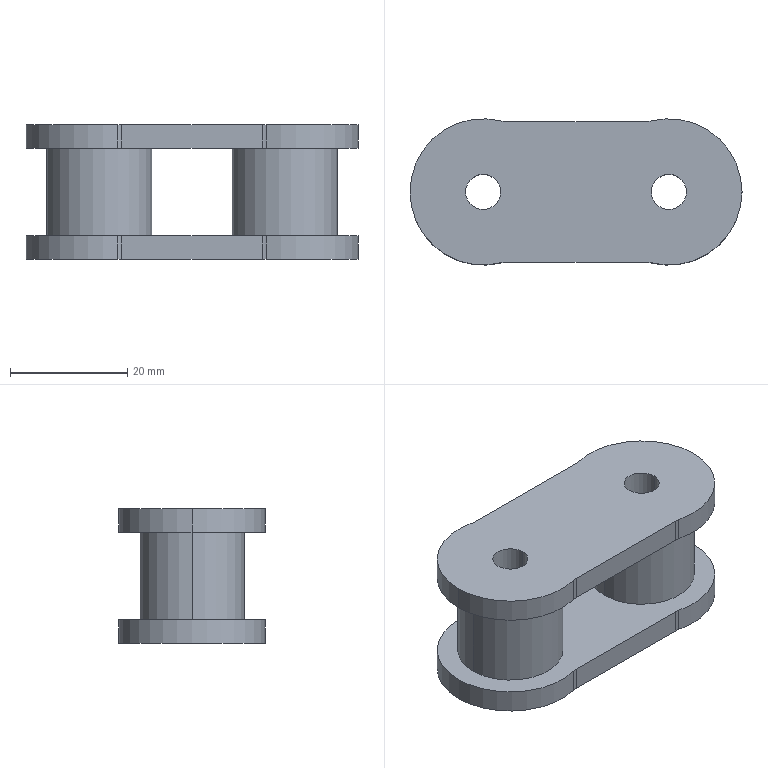Part | STEP file | Motor output chain-06B link 1 | 1 solid | 30 faces | box 56.75 x 25 x 23 mm | volume 16394 mm3 | cylinder 22 | plane 8 | commonest cylinder face diameters 6 x12 25 x6 18 x4
STEP:
#1=CARTESIAN_POINT('',(12.875,0.,-11.5));
#2=VERTEX_POINT('',#1);
#3=CARTESIAN_POINT('',(18.875,0.,-11.5));
#4=VERTEX_POINT('',#3);
#5=CARTESIAN_POINT('',(15.875,0.,-11.5));
#6=DIRECTION('',(0.,0.,1.));
#7=DIRECTION('',(1.,0.,0.));
#8=AXIS2_PLACEMENT_3D('',#5,#6,#7);
#9=CIRCLE('',#8,3.);
#10=EDGE_CURVE('',#2,#4,#9,.T.);
#11=ORIENTED_EDGE('',*,*,#10,.F.);
#12=CARTESIAN_POINT('',(12.875,0.,11.5));
#13=VERTEX_POINT('',#12);
#14=CARTESIAN_POINT('',(12.875,0.,-11.5));
#15=DIRECTION('',(0.,0.,1.));
#16=VECTOR('',#15,1000.);
#17=LINE('',#14,#16);
#18=EDGE_CURVE('',#2,#13,#17,.T.);
#19=ORIENTED_EDGE('',*,*,#18,.T.);
#20=CARTESIAN_POINT('',(18.875,0.,11.5));
#21=VERTEX_POINT('',#20);
#22=CARTESIAN_POINT('',(15.875,0.,11.5));
#23=DIRECTION('',(0.,0.,1.));
#24=DIRECTION('',(1.,0.,0.));
#25=AXIS2_PLACEMENT_3D('',#22,#23,#24);
#26=CIRCLE('',#25,3.);
#27=EDGE_CURVE('',#13,#21,#26,.T.);
#28=ORIENTED_EDGE('',*,*,#27,.T.);
#29=CARTESIAN_POINT('',(18.875,0.,-11.5));
#30=DIRECTION('',(0.,0.,1.));
#31=VECTOR('',#30,1000.);
#32=LINE('',#29,#31);
#33=EDGE_CURVE('',#4,#21,#32,.T.);
#34=ORIENTED_EDGE('',*,*,#33,.F.);
#35=EDGE_LOOP('',(#11,#19,#28,#34));
#36=FACE_OUTER_BOUND('',#35,.T.);
#37=CARTESIAN_POINT('',(15.875,0.,-11.5));
#38=DIRECTION('',(0.,0.,1.));
#39=DIRECTION('',(1.,0.,0.));
#40=AXIS2_PLACEMENT_3D('',#37,#38,#39);
#41=CYLINDRICAL_SURFACE('',#40,3.);
#42=ADVANCED_FACE('',(#36),#41,.F.);
#43=CARTESIAN_POINT('',(-18.875,0.,-11.5));
#44=VERTEX_POINT('',#43);
#45=CARTESIAN_POINT('',(-12.875,0.,-11.5));
#46=VERTEX_POINT('',#45);
#47=CARTESIAN_POINT('',(-15.875,0.,-11.5));
#48=DIRECTION('',(0.,0.,1.));
#49=DIRECTION('',(1.,0.,0.));
#50=AXIS2_PLACEMENT_3D('',#47,#48,#49);
#51=CIRCLE('',#50,3.);
#52=EDGE_CURVE('',#44,#46,#51,.T.);
#53=ORIENTED_EDGE('',*,*,#52,.F.);
#54=CARTESIAN_POINT('',(-18.875,0.,11.5));
#55=VERTEX_POINT('',#54);
#56=CARTESIAN_POINT('',(-18.875,0.,-11.5));
#57=DIRECTION('',(0.,0.,1.));
#58=VECTOR('',#57,1000.);
#59=LINE('',#56,#58);
#60=EDGE_CURVE('',#44,#55,#59,.T.);
#61=ORIENTED_EDGE('',*,*,#60,.T.);
#62=CARTESIAN_POINT('',(-12.875,0.,11.5));
#63=VERTEX_POINT('',#62);
#64=CARTESIAN_POINT('',(-15.875,0.,11.5));
#65=DIRECTION('',(0.,0.,1.));
#66=DIRECTION('',(1.,0.,0.));
#67=AXIS2_PLACEMENT_3D('',#64,#65,#66);
#68=CIRCLE('',#67,3.);
#69=EDGE_CURVE('',#55,#63,#68,.T.);
#70=ORIENTED_EDGE('',*,*,#69,.T.);
#71=CARTESIAN_POINT('',(-12.875,0.,-11.5));
#72=DIRECTION('',(0.,0.,1.));
#73=VECTOR('',#72,1000.);
#74=LINE('',#71,#73);
#75=EDGE_CURVE('',#46,#63,#74,.T.);
#76=ORIENTED_EDGE('',*,*,#75,.F.);
#77=EDGE_LOOP('',(#53,#61,#70,#76));
#78=FACE_OUTER_BOUND('',#77,.T.);
#79=CARTESIAN_POINT('',(-15.875,0.,-11.5));
#80=DIRECTION('',(0.,0.,1.));
#81=DIRECTION('',(1.,0.,0.));
#82=AXIS2_PLACEMENT_3D('',#79,#80,#81);
#83=CYLINDRICAL_SURFACE('',#82,3.);
#84=ADVANCED_FACE('',(#78),#83,.F.);
#85=CARTESIAN_POINT('',(12.726,-12.097,-11.5));
#86=VERTEX_POINT('',#85);
#87=CARTESIAN_POINT('',(28.375,0.,-11.5));
#88=VERTEX_POINT('',#87);
#89=CARTESIAN_POINT('',(15.875,0.,-11.5));
#90=DIRECTION('',(0.,0.,1.));
#91=DIRECTION('',(1.,0.,0.));
#92=AXIS2_PLACEMENT_3D('',#89,#90,#91);
#93=CIRCLE('',#92,12.5);
#94=EDGE_CURVE('',#86,#88,#93,.T.);
#95=ORIENTED_EDGE('',*,*,#94,.T.);
#96=CARTESIAN_POINT('',(28.375,0.,-7.5));
#97=VERTEX_POINT('',#96);
#98=CARTESIAN_POINT('',(28.375,0.,-11.5));
#99=DIRECTION('',(0.,0.,1.));
#100=VECTOR('',#99,1000.);
#101=LINE('',#98,#100);
#102=EDGE_CURVE('',#88,#97,#101,.T.);
#103=ORIENTED_EDGE('',*,*,#102,.T.);
#104=CARTESIAN_POINT('',(12.726,-12.097,-7.5));
#105=VERTEX_POINT('',#104);
#106=CARTESIAN_POINT('',(15.875,0.,-7.5));
#107=DIRECTION('',(0.,0.,1.));
#108=DIRECTION('',(1.,0.,0.));
#109=AXIS2_PLACEMENT_3D('',#106,#107,#108);
#110=CIRCLE('',#109,12.5);
#111=EDGE_CURVE('',#105,#97,#110,.T.);
#112=ORIENTED_EDGE('',*,*,#111,.F.);
#113=CARTESIAN_POINT('',(12.726,-12.097,-11.5));
#114=DIRECTION('',(0.,0.,1.));
#115=VECTOR('',#114,1000.);
#116=LINE('',#113,#115);
#117=EDGE_CURVE('',#86,#105,#116,.T.);
#118=ORIENTED_EDGE('',*,*,#117,.F.);
#119=EDGE_LOOP('',(#95,#103,#112,#118));
#120=FACE_OUTER_BOUND('',#119,.T.);
#121=CARTESIAN_POINT('',(15.875,0.,-11.5));
#122=DIRECTION('',(0.,0.,1.));
#123=DIRECTION('',(1.,0.,0.));
#124=AXIS2_PLACEMENT_3D('',#121,#122,#123);
#125=CYLINDRICAL_SURFACE('',#124,12.5);
#126=ADVANCED_FACE('',(#120),#125,.T.);
#127=CARTESIAN_POINT('',(24.875,0.,7.5));
#128=VERTEX_POINT('',#127);
#129=CARTESIAN_POINT('',(6.875,0.,7.5));
#130=VERTEX_POINT('',#129);
#131=CARTESIAN_POINT('',(15.875,0.,7.5));
#132=DIRECTION('',(0.,0.,1.));
#133=DIRECTION('',(1.,0.,0.));
#134=AXIS2_PLACEMENT_3D('',#131,#132,#133);
#135=CIRCLE('',#134,9.);
#136=EDGE_CURVE('',#128,#130,#135,.T.);
#137=ORIENTED_EDGE('',*,*,#136,.F.);
#138=CARTESIAN_POINT('',(24.875,0.,-7.5));
#139=VERTEX_POINT('',#138);
#140=CARTESIAN_POINT('',(24.875,0.,7.5));
#141=DIRECTION('',(0.,0.,-1.));
#142=VECTOR('',#141,1000.);
#143=LINE('',#140,#142);
#144=EDGE_CURVE('',#128,#139,#143,.T.);
#145=ORIENTED_EDGE('',*,*,#144,.T.);
#146=CARTESIAN_POINT('',(6.875,0.,-7.5));
#147=VERTEX_POINT('',#146);
#148=CARTESIAN_POINT('',(15.875,0.,-7.5));
#149=DIRECTION('',(0.,0.,1.));
#150=DIRECTION('',(1.,0.,0.));
#151=AXIS2_PLACEMENT_3D('',#148,#149,#150);
#152=CIRCLE('',#151,9.);
#153=EDGE_CURVE('',#139,#147,#152,.T.);
#154=ORIENTED_EDGE('',*,*,#153,.T.);
#155=CARTESIAN_POINT('',(6.875,0.,7.5));
#156=DIRECTION('',(0.,0.,-1.));
#157=VECTOR('',#156,1000.);
#158=LINE('',#155,#157);
#159=EDGE_CURVE('',#130,#147,#158,.T.);
#160=ORIENTED_EDGE('',*,*,#159,.F.);
#161=EDGE_LOOP('',(#137,#145,#154,#160));
#162=FACE_OUTER_BOUND('',#161,.T.);
#163=CARTESIAN_POINT('',(15.875,0.,7.5));
#164=DIRECTION('',(0.,0.,-1.));
#165=DIRECTION('',(-1.,0.,0.));
#166=AXIS2_PLACEMENT_3D('',#163,#164,#165);
#167=CYLINDRICAL_SURFACE('',#166,9.);
#168=ADVANCED_FACE('',(#162),#167,.T.);
#169=CARTESIAN_POINT('',(-28.375,0.,11.5));
#170=VERTEX_POINT('',#169);
#171=CARTESIAN_POINT('',(-12.726,-12.097,11.5));
#172=VERTEX_POINT('',#171);
#173=CARTESIAN_POINT('',(-15.875,0.,11.5));
#174=DIRECTION('',(0.,0.,1.));
#175=DIRECTION('',(1.,0.,0.));
#176=AXIS2_PLACEMENT_3D('',#173,#174,#175);
#177=CIRCLE('',#176,12.5);
#178=EDGE_CURVE('',#170,#172,#177,.T.);
#179=ORIENTED_EDGE('',*,*,#178,.F.);
#180=CARTESIAN_POINT('',(-28.375,0.,7.5));
#181=VERTEX_POINT('',#180);
#182=CARTESIAN_POINT('',(-28.375,0.,11.5));
#183=DIRECTION('',(0.,0.,-1.));
#184=VECTOR('',#183,1000.);
#185=LINE('',#182,#184);
#186=EDGE_CURVE('',#170,#181,#185,.T.);
#187=ORIENTED_EDGE('',*,*,#186,.T.);
#188=CARTESIAN_POINT('',(-12.726,-12.097,7.5));
#189=VERTEX_POINT('',#188);
#190=CARTESIAN_POINT('',(-15.875,0.,7.5));
#191=DIRECTION('',(0.,0.,1.));
#192=DIRECTION('',(1.,0.,0.));
#193=AXIS2_PLACEMENT_3D('',#190,#191,#192);
#194=CIRCLE('',#193,12.5);
#195=EDGE_CURVE('',#181,#189,#194,.T.);
#196=ORIENTED_EDGE('',*,*,#195,.T.);
#197=CARTESIAN_POINT('',(-12.726,-12.097,11.5));
#198=DIRECTION('',(0.,0.,-1.));
#199=VECTOR('',#198,1000.);
#200=LINE('',#197,#199);
#201=EDGE_CURVE('',#172,#189,#200,.T.);
#202=ORIENTED_EDGE('',*,*,#201,.F.);
#203=EDGE_LOOP('',(#179,#187,#196,#202));
#204=FACE_OUTER_BOUND('',#203,.T.);
#205=CARTESIAN_POINT('',(-15.875,0.,11.5));
#206=DIRECTION('',(0.,0.,-1.));
#207=DIRECTION('',(-1.,0.,0.));
#208=AXIS2_PLACEMENT_3D('',#205,#206,#207);
#209=CYLINDRICAL_SURFACE('',#208,12.5);
#210=ADVANCED_FACE('',(#204),#209,.T.);
#211=CARTESIAN_POINT('',(-6.875,0.,7.5));
#212=VERTEX_POINT('',#211);
#213=CARTESIAN_POINT('',(-24.875,0.,7.5));
#214=VERTEX_POINT('',#213);
#215=CARTESIAN_POINT('',(-15.875,0.,7.5));
#216=DIRECTION('',(0.,0.,1.));
#217=DIRECTION('',(1.,0.,0.));
#218=AXIS2_PLACEMENT_3D('',#215,#216,#217);
#219=CIRCLE('',#218,9.);
#220=EDGE_CURVE('',#212,#214,#219,.T.);
#221=ORIENTED_EDGE('',*,*,#220,.F.);
#222=CARTESIAN_POINT('',(-6.875,0.,-7.5));
#223=VERTEX_POINT('',#222);
#224=CARTESIAN_POINT('',(-6.875,0.,7.5));
#225=DIRECTION('',(0.,0.,-1.));
#226=VECTOR('',#225,1000.);
#227=LINE('',#224,#226);
#228=EDGE_CURVE('',#212,#223,#227,.T.);
#229=ORIENTED_EDGE('',*,*,#228,.T.);
#230=CARTESIAN_POINT('',(-24.875,0.,-7.5));
#231=VERTEX_POINT('',#230);
#232=CARTESIAN_POINT('',(-15.875,0.,-7.5));
#233=DIRECTION('',(0.,0.,1.));
#234=DIRECTION('',(1.,0.,0.));
#235=AXIS2_PLACEMENT_3D('',#232,#233,#234);
#236=CIRCLE('',#235,9.);
#237=EDGE_CURVE('',#223,#231,#236,.T.);
#238=ORIENTED_EDGE('',*,*,#237,.T.);
#239=CARTESIAN_POINT('',(-24.875,0.,7.5));
#240=DIRECTION('',(0.,0.,-1.));
#241=VECTOR('',#240,1000.);
#242=LINE('',#239,#241);
#243=EDGE_CURVE('',#214,#231,#242,.T.);
#244=ORIENTED_EDGE('',*,*,#243,.F.);
#245=EDGE_LOOP('',(#221,#229,#238,#244));
#246=FACE_OUTER_BOUND('',#245,.T.);
#247=CARTESIAN_POINT('',(-15.875,0.,7.5));
#248=DIRECTION('',(0.,0.,-1.));
#249=DIRECTION('',(-1.,0.,0.));
#250=AXIS2_PLACEMENT_3D('',#247,#248,#249);
#251=CYLINDRICAL_SURFACE('',#250,9.);
#252=ADVANCED_FACE('',(#246),#251,.T.);
#253=ORIENTED_EDGE('',*,*,#228,.F.);
#254=CARTESIAN_POINT('',(-15.875,0.,7.5));
#255=DIRECTION('',(0.,0.,1.));
#256=DIRECTION('',(1.,0.,0.));
#257=AXIS2_PLACEMENT_3D('',#254,#255,#256);
#258=CIRCLE('',#257,9.);
#259=EDGE_CURVE('',#214,#212,#258,.T.);
#260=ORIENTED_EDGE('',*,*,#259,.F.);
#261=ORIENTED_EDGE('',*,*,#243,.T.);
#262=CARTESIAN_POINT('',(-15.875,0.,-7.5));
#263=DIRECTION('',(0.,0.,1.));
#264=DIRECTION('',(1.,0.,0.));
#265=AXIS2_PLACEMENT_3D('',#262,#263,#264);
#266=CIRCLE('',#265,9.);
#267=EDGE_CURVE('',#231,#223,#266,.T.);
#268=ORIENTED_EDGE('',*,*,#267,.T.);
#269=EDGE_LOOP('',(#253,#260,#261,#268));
#270=FACE_OUTER_BOUND('',#269,.T.);
#271=CARTESIAN_POINT('',(-15.875,0.,7.5));
#272=DIRECTION('',(0.,0.,-1.));
#273=DIRECTION('',(-1.,0.,0.));
#274=AXIS2_PLACEMENT_3D('',#271,#272,#273);
#275=CYLINDRICAL_SURFACE('',#274,9.);
#276=ADVANCED_FACE('',(#270),#275,.T.);
#277=CARTESIAN_POINT('',(11.97,-12.,7.5));
#278=VERTEX_POINT('',#277);
#279=CARTESIAN_POINT('',(12.726,-12.097,7.5));
#280=VERTEX_POINT('',#279);
#281=CARTESIAN_POINT('',(11.97,-15.,7.5));
#282=DIRECTION('',(0.,0.,-1.));
#283=DIRECTION('',(-1.,0.,0.));
#284=AXIS2_PLACEMENT_3D('',#281,#282,#283);
#285=CIRCLE('',#284,3.);
#286=EDGE_CURVE('',#278,#280,#285,.T.);
#287=ORIENTED_EDGE('',*,*,#286,.T.);
#288=CARTESIAN_POINT('',(12.726,-12.097,11.5));
#289=VERTEX_POINT('',#288);
#290=CARTESIAN_POINT('',(12.726,-12.097,11.5));
#291=DIRECTION('',(0.,0.,-1.));
#292=VECTOR('',#291,1000.);
#293=LINE('',#290,#292);
#294=EDGE_CURVE('',#289,#280,#293,.T.);
#295=ORIENTED_EDGE('',*,*,#294,.F.);
#296=CARTESIAN_POINT('',(11.97,-12.,11.5));
#297=VERTEX_POINT('',#296);
#298=CARTESIAN_POINT('',(11.97,-15.,11.5));
#299=DIRECTION('',(0.,0.,-1.));
#300=DIRECTION('',(-1.,0.,0.));
#301=AXIS2_PLACEMENT_3D('',#298,#299,#300);
#302=CIRCLE('',#301,3.);
#303=EDGE_CURVE('',#297,#289,#302,.T.);
#304=ORIENTED_EDGE('',*,*,#303,.F.);
#305=CARTESIAN_POINT('',(11.97,-12.,11.5));
#306=DIRECTION('',(0.,0.,-1.));
#307=VECTOR('',#306,1000.);
#308=LINE('',#305,#307);
#309=EDGE_CURVE('',#297,#278,#308,.T.);
#310=ORIENTED_EDGE('',*,*,#309,.T.);
#311=EDGE_LOOP('',(#287,#295,#304,#310));
#312=FACE_OUTER_BOUND('',#311,.T.);
#313=CARTESIAN_POINT('',(11.97,-15.,11.5));
#314=DIRECTION('',(0.,0.,-1.));
#315=DIRECTION('',(-1.,0.,0.));
#316=AXIS2_PLACEMENT_3D('',#313,#314,#315);
#317=CYLINDRICAL_SURFACE('',#316,3.);
#318=ADVANCED_FACE('',(#312),#317,.F.);
#319=CARTESIAN_POINT('',(12.726,12.097,7.5));
#320=VERTEX_POINT('',#319);
#321=CARTESIAN_POINT('',(15.875,0.,7.5));
#322=DIRECTION('',(0.,0.,1.));
#323=DIRECTION('',(1.,0.,0.));
#324=AXIS2_PLACEMENT_3D('',#321,#322,#323);
#325=CIRCLE('',#324,12.5);
#326=EDGE_CURVE('',#280,#320,#325,.T.);
#327=ORIENTED_EDGE('',*,*,#326,.T.);
#328=CARTESIAN_POINT('',(12.726,12.097,11.5));
#329=VERTEX_POINT('',#328);
#330=CARTESIAN_POINT('',(12.726,12.097,11.5));
#331=DIRECTION('',(0.,0.,-1.));
#332=VECTOR('',#331,1000.);
#333=LINE('',#330,#332);
#334=EDGE_CURVE('',#329,#320,#333,.T.);
#335=ORIENTED_EDGE('',*,*,#334,.F.);
#336=CARTESIAN_POINT('',(15.875,0.,11.5));
#337=DIRECTION('',(0.,0.,1.));
#338=DIRECTION('',(1.,0.,0.));
#339=AXIS2_PLACEMENT_3D('',#336,#337,#338);
#340=CIRCLE('',#339,12.5);
#341=EDGE_CURVE('',#289,#329,#340,.T.);
#342=ORIENTED_EDGE('',*,*,#341,.F.);
#343=ORIENTED_EDGE('',*,*,#294,.T.);
#344=EDGE_LOOP('',(#327,#335,#342,#343));
#345=FACE_OUTER_BOUND('',#344,.T.);
#346=CARTESIAN_POINT('',(15.875,0.,11.5));
#347=DIRECTION('',(0.,0.,-1.));
#348=DIRECTION('',(-1.,0.,0.));
#349=AXIS2_PLACEMENT_3D('',#346,#347,#348);
#350=CYLINDRICAL_SURFACE('',#349,12.5);
#351=ADVANCED_FACE('',(#345),#350,.T.);
#352=CARTESIAN_POINT('',(11.97,12.,7.5));
#353=VERTEX_POINT('',#352);
#354=CARTESIAN_POINT('',(11.97,15.,7.5));
#355=DIRECTION('',(0.,0.,-1.));
#356=DIRECTION('',(1.,0.,0.));
#357=AXIS2_PLACEMENT_3D('',#354,#355,#356);
#358=CIRCLE('',#357,3.);
#359=EDGE_CURVE('',#320,#353,#358,.T.);
#360=ORIENTED_EDGE('',*,*,#359,.T.);
#361=CARTESIAN_POINT('',(11.97,12.,11.5));
#362=VERTEX_POINT('',#361);
#363=CARTESIAN_POINT('',(11.97,12.,11.5));
#364=DIRECTION('',(0.,0.,-1.));
#365=VECTOR('',#364,1000.);
#366=LINE('',#363,#365);
#367=EDGE_CURVE('',#362,#353,#366,.T.);
#368=ORIENTED_EDGE('',*,*,#367,.F.);
#369=CARTESIAN_POINT('',(11.97,15.,11.5));
#370=DIRECTION('',(0.,0.,-1.));
#371=DIRECTION('',(1.,0.,0.));
#372=AXIS2_PLACEMENT_3D('',#369,#370,#371);
#373=CIRCLE('',#372,3.);
#374=EDGE_CURVE('',#329,#362,#373,.T.);
#375=ORIENTED_EDGE('',*,*,#374,.F.);
#376=ORIENTED_EDGE('',*,*,#334,.T.);
#377=EDGE_LOOP('',(#360,#368,#375,#376));
#378=FACE_OUTER_BOUND('',#377,.T.);
#379=CARTESIAN_POINT('',(11.97,15.,11.5));
#380=DIRECTION('',(0.,0.,-1.));
#381=DIRECTION('',(-1.,0.,0.));
#382=AXIS2_PLACEMENT_3D('',#379,#380,#381);
#383=CYLINDRICAL_SURFACE('',#382,3.);
#384=ADVANCED_FACE('',(#378),#383,.F.);
#385=CARTESIAN_POINT('',(-11.97,12.,7.5));
#386=VERTEX_POINT('',#385);
#387=CARTESIAN_POINT('',(-11.97,12.,7.5));
#388=DIRECTION('',(-1.,0.,0.));
#389=VECTOR('',#388,1000.);
#390=LINE('',#387,#389);
#391=EDGE_CURVE('',#353,#386,#390,.T.);
#392=ORIENTED_EDGE('',*,*,#391,.T.);
#393=CARTESIAN_POINT('',(-11.97,12.,11.5));
#394=VERTEX_POINT('',#393);
#395=CARTESIAN_POINT('',(-11.97,12.,11.5));
#396=DIRECTION('',(0.,0.,-1.));
#397=VECTOR('',#396,1000.);
#398=LINE('',#395,#397);
#399=EDGE_CURVE('',#394,#386,#398,.T.);
#400=ORIENTED_EDGE('',*,*,#399,.F.);
#401=CARTESIAN_POINT('',(-11.97,12.,11.5));
#402=DIRECTION('',(-1.,0.,0.));
#403=VECTOR('',#402,1000.);
#404=LINE('',#401,#403);
#405=EDGE_CURVE('',#362,#394,#404,.T.);
#406=ORIENTED_EDGE('',*,*,#405,.F.);
#407=ORIENTED_EDGE('',*,*,#367,.T.);
#408=EDGE_LOOP('',(#392,#400,#406,#407));
#409=FACE_OUTER_BOUND('',#408,.T.);
#410=CARTESIAN_POINT('',(-11.97,12.,11.5));
#411=DIRECTION('',(0.,-1.,0.));
#412=DIRECTION('',(0.,0.,-1.));
#413=AXIS2_PLACEMENT_3D('',#410,#411,#412);
#414=PLANE('',#413);
#415=ADVANCED_FACE('',(#409),#414,.F.);
#416=CARTESIAN_POINT('',(-12.726,12.097,7.5));
#417=VERTEX_POINT('',#416);
#418=CARTESIAN_POINT('',(-11.97,15.,7.5));
#419=DIRECTION('',(0.,0.,-1.));
#420=DIRECTION('',(-1.,0.,0.));
#421=AXIS2_PLACEMENT_3D('',#418,#419,#420);
#422=CIRCLE('',#421,3.);
#423=EDGE_CURVE('',#386,#417,#422,.T.);
#424=ORIENTED_EDGE('',*,*,#423,.T.);
#425=CARTESIAN_POINT('',(-12.726,12.097,11.5));
#426=VERTEX_POINT('',#425);
#427=CARTESIAN_POINT('',(-12.726,12.097,11.5));
#428=DIRECTION('',(0.,0.,-1.));
#429=VECTOR('',#428,1000.);
#430=LINE('',#427,#429);
#431=EDGE_CURVE('',#426,#417,#430,.T.);
#432=ORIENTED_EDGE('',*,*,#431,.F.);
#433=CARTESIAN_POINT('',(-11.97,15.,11.5));
#434=DIRECTION('',(0.,0.,-1.));
#435=DIRECTION('',(-1.,0.,0.));
#436=AXIS2_PLACEMENT_3D('',#433,#434,#435);
#437=CIRCLE('',#436,3.);
#438=EDGE_CURVE('',#394,#426,#437,.T.);
#439=ORIENTED_EDGE('',*,*,#438,.F.);
#440=ORIENTED_EDGE('',*,*,#399,.T.);
#441=EDGE_LOOP('',(#424,#432,#439,#440));
#442=FACE_OUTER_BOUND('',#441,.T.);
#443=CARTESIAN_POINT('',(-11.97,15.,11.5));
#444=DIRECTION('',(0.,0.,-1.));
#445=DIRECTION('',(-1.,0.,0.));
#446=AXIS2_PLACEMENT_3D('',#443,#444,#445);
#447=CYLINDRICAL_SURFACE('',#446,3.);
#448=ADVANCED_FACE('',(#442),#447,.F.);
#449=ORIENTED_EDGE('',*,*,#186,.F.);
#450=CARTESIAN_POINT('',(-15.875,0.,11.5));
#451=DIRECTION('',(0.,0.,1.));
#452=DIRECTION('',(1.,0.,0.));
#453=AXIS2_PLACEMENT_3D('',#450,#451,#452);
#454=CIRCLE('',#453,12.5);
#455=EDGE_CURVE('',#426,#170,#454,.T.);
#456=ORIENTED_EDGE('',*,*,#455,.F.);
#457=ORIENTED_EDGE('',*,*,#431,.T.);
#458=CARTESIAN_POINT('',(-15.875,0.,7.5));
#459=DIRECTION('',(0.,0.,1.));
#460=DIRECTION('',(1.,0.,0.));
#461=AXIS2_PLACEMENT_3D('',#458,#459,#460);
#462=CIRCLE('',#461,12.5);
#463=EDGE_CURVE('',#417,#181,#462,.T.);
#464=ORIENTED_EDGE('',*,*,#463,.T.);
#465=EDGE_LOOP('',(#449,#456,#457,#464));
#466=FACE_OUTER_BOUND('',#465,.T.);
#467=CARTESIAN_POINT('',(-15.875,0.,11.5));
#468=DIRECTION('',(0.,0.,-1.));
#469=DIRECTION('',(-1.,0.,0.));
#470=AXIS2_PLACEMENT_3D('',#467,#468,#469);
#471=CYLINDRICAL_SURFACE('',#470,12.5);
#472=ADVANCED_FACE('',(#466),#471,.T.);
#473=CARTESIAN_POINT('',(-11.97,-12.,7.5));
#474=VERTEX_POINT('',#473);
#475=CARTESIAN_POINT('',(-11.97,-15.,7.5));
#476=DIRECTION('',(0.,0.,-1.));
#477=DIRECTION('',(1.,0.,0.));
#478=AXIS2_PLACEMENT_3D('',#475,#476,#477);
#479=CIRCLE('',#478,3.);
#480=EDGE_CURVE('',#189,#474,#479,.T.);
#481=ORIENTED_EDGE('',*,*,#480,.T.);
#482=CARTESIAN_POINT('',(-11.97,-12.,11.5));
#483=VERTEX_POINT('',#482);
#484=CARTESIAN_POINT('',(-11.97,-12.,11.5));
#485=DIRECTION('',(0.,0.,-1.));
#486=VECTOR('',#485,1000.);
#487=LINE('',#484,#486);
#488=EDGE_CURVE('',#483,#474,#487,.T.);
#489=ORIENTED_EDGE('',*,*,#488,.F.);
#490=CARTESIAN_POINT('',(-11.97,-15.,11.5));
#491=DIRECTION('',(0.,0.,-1.));
#492=DIRECTION('',(1.,0.,0.));
#493=AXIS2_PLACEMENT_3D('',#490,#491,#492);
#494=CIRCLE('',#493,3.);
#495=EDGE_CURVE('',#172,#483,#494,.T.);
#496=ORIENTED_EDGE('',*,*,#495,.F.);
#497=ORIENTED_EDGE('',*,*,#201,.T.);
#498=EDGE_LOOP('',(#481,#489,#496,#497));
#499=FACE_OUTER_BOUND('',#498,.T.);
#500=CARTESIAN_POINT('',(-11.97,-15.,11.5));
#501=DIRECTION('',(0.,0.,-1.));
#502=DIRECTION('',(-1.,0.,0.));
#503=AXIS2_PLACEMENT_3D('',#500,#501,#502);
#504=CYLINDRICAL_SURFACE('',#503,3.);
#505=ADVANCED_FACE('',(#499),#504,.F.);
#506=CARTESIAN_POINT('',(-11.97,-12.,7.5));
#507=DIRECTION('',(1.,0.,0.));
#508=VECTOR('',#507,1000.);
#509=LINE('',#506,#508);
#510=EDGE_CURVE('',#474,#278,#509,.T.);
#511=ORIENTED_EDGE('',*,*,#510,.T.);
#512=ORIENTED_EDGE('',*,*,#309,.F.);
#513=CARTESIAN_POINT('',(-11.97,-12.,11.5));
#514=DIRECTION('',(1.,0.,0.));
#515=VECTOR('',#514,1000.);
#516=LINE('',#513,#515);
#517=EDGE_CURVE('',#483,#297,#516,.T.);
#518=ORIENTED_EDGE('',*,*,#517,.F.);
#519=ORIENTED_EDGE('',*,*,#488,.T.);
#520=EDGE_LOOP('',(#511,#512,#518,#519));
#521=FACE_OUTER_BOUND('',#520,.T.);
#522=CARTESIAN_POINT('',(-11.97,-12.,11.5));
#523=DIRECTION('',(0.,1.,0.));
#524=DIRECTION('',(0.,0.,1.));
#525=AXIS2_PLACEMENT_3D('',#522,#523,#524);
#526=PLANE('',#525);
#527=ADVANCED_FACE('',(#521),#526,.F.);
#528=CARTESIAN_POINT('',(15.875,0.,11.5));
#529=DIRECTION('',(0.,0.,1.));
#530=DIRECTION('',(1.,0.,0.));
#531=AXIS2_PLACEMENT_3D('',#528,#529,#530);
#532=CIRCLE('',#531,3.);
#533=EDGE_CURVE('',#21,#13,#532,.T.);
#534=ORIENTED_EDGE('',*,*,#533,.F.);
#535=ORIENTED_EDGE('',*,*,#27,.F.);
#536=EDGE_LOOP('',(#534,#535));
#537=FACE_BOUND('',#536,.T.);
#538=CARTESIAN_POINT('',(-15.875,0.,11.5));
#539=DIRECTION('',(0.,0.,1.));
#540=DIRECTION('',(1.,0.,0.));
#541=AXIS2_PLACEMENT_3D('',#538,#539,#540);
#542=CIRCLE('',#541,3.);
#543=EDGE_CURVE('',#63,#55,#542,.T.);
#544=ORIENTED_EDGE('',*,*,#543,.F.);
#545=ORIENTED_EDGE('',*,*,#69,.F.);
#546=EDGE_LOOP('',(#544,#545));
#547=FACE_BOUND('',#546,.T.);
#548=ORIENTED_EDGE('',*,*,#303,.T.);
#549=ORIENTED_EDGE('',*,*,#341,.T.);
#550=ORIENTED_EDGE('',*,*,#374,.T.);
#551=ORIENTED_EDGE('',*,*,#405,.T.);
#552=ORIENTED_EDGE('',*,*,#438,.T.);
#553=ORIENTED_EDGE('',*,*,#455,.T.);
#554=ORIENTED_EDGE('',*,*,#178,.T.);
#555=ORIENTED_EDGE('',*,*,#495,.T.);
#556=ORIENTED_EDGE('',*,*,#517,.T.);
#557=EDGE_LOOP('',(#548,#549,#550,#551,#552,#553,#554,#555,#556));
#558=FACE_OUTER_BOUND('',#557,.T.);
#559=CARTESIAN_POINT('',(11.97,-15.,11.5));
#560=DIRECTION('',(0.,0.,-1.));
#561=DIRECTION('',(-1.,0.,0.));
#562=AXIS2_PLACEMENT_3D('',#559,#560,#561);
#563=PLANE('',#562);
#564=ADVANCED_FACE('',(#537,#547,#558),#563,.F.);
#565=CARTESIAN_POINT('',(15.875,0.,7.5));
#566=DIRECTION('',(0.,0.,1.));
#567=DIRECTION('',(1.,0.,0.));
#568=AXIS2_PLACEMENT_3D('',#565,#566,#567);
#569=CIRCLE('',#568,9.);
#570=EDGE_CURVE('',#130,#128,#569,.T.);
#571=ORIENTED_EDGE('',*,*,#570,.T.);
#572=ORIENTED_EDGE('',*,*,#136,.T.);
#573=EDGE_LOOP('',(#571,#572));
#574=FACE_BOUND('',#573,.T.);
#575=ORIENTED_EDGE('',*,*,#259,.T.);
#576=ORIENTED_EDGE('',*,*,#220,.T.);
#577=EDGE_LOOP('',(#575,#576));
#578=FACE_BOUND('',#577,.T.);
#579=ORIENTED_EDGE('',*,*,#286,.F.);
#580=ORIENTED_EDGE('',*,*,#510,.F.);
#581=ORIENTED_EDGE('',*,*,#480,.F.);
#582=ORIENTED_EDGE('',*,*,#195,.F.);
#583=ORIENTED_EDGE('',*,*,#463,.F.);
#584=ORIENTED_EDGE('',*,*,#423,.F.);
#585=ORIENTED_EDGE('',*,*,#391,.F.);
#586=ORIENTED_EDGE('',*,*,#359,.F.);
#587=ORIENTED_EDGE('',*,*,#326,.F.);
#588=EDGE_LOOP('',(#579,#580,#581,#582,#583,#584,#585,#586,#587));
#589=FACE_OUTER_BOUND('',#588,.T.);
#590=CARTESIAN_POINT('',(11.97,-15.,7.5));
#591=DIRECTION('',(0.,0.,-1.));
#592=DIRECTION('',(-1.,0.,0.));
#593=AXIS2_PLACEMENT_3D('',#590,#591,#592);
#594=PLANE('',#593);
#595=ADVANCED_FACE('',(#574,#578,#589),#594,.T.);
#596=ORIENTED_EDGE('',*,*,#144,.F.);
#597=ORIENTED_EDGE('',*,*,#570,.F.);
#598=ORIENTED_EDGE('',*,*,#159,.T.);
#599=CARTESIAN_POINT('',(15.875,0.,-7.5));
#600=DIRECTION('',(0.,0.,1.));
#601=DIRECTION('',(1.,0.,0.));
#602=AXIS2_PLACEMENT_3D('',#599,#600,#601);
#603=CIRCLE('',#602,9.);
#604=EDGE_CURVE('',#147,#139,#603,.T.);
#605=ORIENTED_EDGE('',*,*,#604,.T.);
#606=EDGE_LOOP('',(#596,#597,#598,#605));
#607=FACE_OUTER_BOUND('',#606,.T.);
#608=CARTESIAN_POINT('',(15.875,0.,7.5));
#609=DIRECTION('',(0.,0.,-1.));
#610=DIRECTION('',(-1.,0.,0.));
#611=AXIS2_PLACEMENT_3D('',#608,#609,#610);
#612=CYLINDRICAL_SURFACE('',#611,9.);
#613=ADVANCED_FACE('',(#607),#612,.T.);
#614=CARTESIAN_POINT('',(11.97,-12.,-7.5));
#615=VERTEX_POINT('',#614);
#616=CARTESIAN_POINT('',(11.97,-15.,-7.5));
#617=DIRECTION('',(0.,0.,-1.));
#618=DIRECTION('',(-1.,0.,0.));
#619=AXIS2_PLACEMENT_3D('',#616,#617,#618);
#620=CIRCLE('',#619,3.);
#621=EDGE_CURVE('',#615,#105,#620,.T.);
#622=ORIENTED_EDGE('',*,*,#621,.F.);
#623=CARTESIAN_POINT('',(11.97,-12.,-11.5));
#624=VERTEX_POINT('',#623);
#625=CARTESIAN_POINT('',(11.97,-12.,-11.5));
#626=DIRECTION('',(0.,0.,1.));
#627=VECTOR('',#626,1000.);
#628=LINE('',#625,#627);
#629=EDGE_CURVE('',#624,#615,#628,.T.);
#630=ORIENTED_EDGE('',*,*,#629,.F.);
#631=CARTESIAN_POINT('',(11.97,-15.,-11.5));
#632=DIRECTION('',(0.,0.,-1.));
#633=DIRECTION('',(-1.,0.,0.));
#634=AXIS2_PLACEMENT_3D('',#631,#632,#633);
#635=CIRCLE('',#634,3.);
#636=EDGE_CURVE('',#624,#86,#635,.T.);
#637=ORIENTED_EDGE('',*,*,#636,.T.);
#638=ORIENTED_EDGE('',*,*,#117,.T.);
#639=EDGE_LOOP('',(#622,#630,#637,#638));
#640=FACE_OUTER_BOUND('',#639,.T.);
#641=CARTESIAN_POINT('',(11.97,-15.,-11.5));
#642=DIRECTION('',(0.,0.,1.));
#643=DIRECTION('',(1.,0.,0.));
#644=AXIS2_PLACEMENT_3D('',#641,#642,#643);
#645=CYLINDRICAL_SURFACE('',#644,3.);
#646=ADVANCED_FACE('',(#640),#645,.F.);
#647=CARTESIAN_POINT('',(-11.97,-12.,-7.5));
#648=VERTEX_POINT('',#647);
#649=CARTESIAN_POINT('',(-11.97,-12.,-7.5));
#650=DIRECTION('',(1.,0.,0.));
#651=VECTOR('',#650,1000.);
#652=LINE('',#649,#651);
#653=EDGE_CURVE('',#648,#615,#652,.T.);
#654=ORIENTED_EDGE('',*,*,#653,.F.);
#655=CARTESIAN_POINT('',(-11.97,-12.,-11.5));
#656=VERTEX_POINT('',#655);
#657=CARTESIAN_POINT('',(-11.97,-12.,-11.5));
#658=DIRECTION('',(0.,0.,1.));
#659=VECTOR('',#658,1000.);
#660=LINE('',#657,#659);
#661=EDGE_CURVE('',#656,#648,#660,.T.);
#662=ORIENTED_EDGE('',*,*,#661,.F.);
#663=CARTESIAN_POINT('',(-11.97,-12.,-11.5));
#664=DIRECTION('',(1.,0.,0.));
#665=VECTOR('',#664,1000.);
#666=LINE('',#663,#665);
#667=EDGE_CURVE('',#656,#624,#666,.T.);
#668=ORIENTED_EDGE('',*,*,#667,.T.);
#669=ORIENTED_EDGE('',*,*,#629,.T.);
#670=EDGE_LOOP('',(#654,#662,#668,#669));
#671=FACE_OUTER_BOUND('',#670,.T.);
#672=CARTESIAN_POINT('',(-11.97,-12.,-11.5));
#673=DIRECTION('',(0.,-1.,0.));
#674=DIRECTION('',(0.,0.,-1.));
#675=AXIS2_PLACEMENT_3D('',#672,#673,#674);
#676=PLANE('',#675);
#677=ADVANCED_FACE('',(#671),#676,.T.);
#678=CARTESIAN_POINT('',(-12.726,-12.097,-7.5));
#679=VERTEX_POINT('',#678);
#680=CARTESIAN_POINT('',(-11.97,-15.,-7.5));
#681=DIRECTION('',(0.,0.,-1.));
#682=DIRECTION('',(1.,0.,0.));
#683=AXIS2_PLACEMENT_3D('',#680,#681,#682);
#684=CIRCLE('',#683,3.);
#685=EDGE_CURVE('',#679,#648,#684,.T.);
#686=ORIENTED_EDGE('',*,*,#685,.F.);
#687=CARTESIAN_POINT('',(-12.726,-12.097,-11.5));
#688=VERTEX_POINT('',#687);
#689=CARTESIAN_POINT('',(-12.726,-12.097,-11.5));
#690=DIRECTION('',(0.,0.,1.));
#691=VECTOR('',#690,1000.);
#692=LINE('',#689,#691);
#693=EDGE_CURVE('',#688,#679,#692,.T.);
#694=ORIENTED_EDGE('',*,*,#693,.F.);
#695=CARTESIAN_POINT('',(-11.97,-15.,-11.5));
#696=DIRECTION('',(0.,0.,-1.));
#697=DIRECTION('',(1.,0.,0.));
#698=AXIS2_PLACEMENT_3D('',#695,#696,#697);
#699=CIRCLE('',#698,3.);
#700=EDGE_CURVE('',#688,#656,#699,.T.);
#701=ORIENTED_EDGE('',*,*,#700,.T.);
#702=ORIENTED_EDGE('',*,*,#661,.T.);
#703=EDGE_LOOP('',(#686,#694,#701,#702));
#704=FACE_OUTER_BOUND('',#703,.T.);
#705=CARTESIAN_POINT('',(-11.97,-15.,-11.5));
#706=DIRECTION('',(0.,0.,1.));
#707=DIRECTION('',(1.,0.,0.));
#708=AXIS2_PLACEMENT_3D('',#705,#706,#707);
#709=CYLINDRICAL_SURFACE('',#708,3.);
#710=ADVANCED_FACE('',(#704),#709,.F.);
#711=CARTESIAN_POINT('',(-12.726,12.097,-7.5));
#712=VERTEX_POINT('',#711);
#713=CARTESIAN_POINT('',(-15.875,0.,-7.5));
#714=DIRECTION('',(0.,0.,1.));
#715=DIRECTION('',(1.,0.,0.));
#716=AXIS2_PLACEMENT_3D('',#713,#714,#715);
#717=CIRCLE('',#716,12.5);
#718=EDGE_CURVE('',#712,#679,#717,.T.);
#719=ORIENTED_EDGE('',*,*,#718,.F.);
#720=CARTESIAN_POINT('',(-12.726,12.097,-11.5));
#721=VERTEX_POINT('',#720);
#722=CARTESIAN_POINT('',(-12.726,12.097,-11.5));
#723=DIRECTION('',(0.,0.,1.));
#724=VECTOR('',#723,1000.);
#725=LINE('',#722,#724);
#726=EDGE_CURVE('',#721,#712,#725,.T.);
#727=ORIENTED_EDGE('',*,*,#726,.F.);
#728=CARTESIAN_POINT('',(-15.875,0.,-11.5));
#729=DIRECTION('',(0.,0.,1.));
#730=DIRECTION('',(1.,0.,0.));
#731=AXIS2_PLACEMENT_3D('',#728,#729,#730);
#732=CIRCLE('',#731,12.5);
#733=EDGE_CURVE('',#721,#688,#732,.T.);
#734=ORIENTED_EDGE('',*,*,#733,.T.);
#735=ORIENTED_EDGE('',*,*,#693,.T.);
#736=EDGE_LOOP('',(#719,#727,#734,#735));
#737=FACE_OUTER_BOUND('',#736,.T.);
#738=CARTESIAN_POINT('',(-15.875,0.,-11.5));
#739=DIRECTION('',(0.,0.,1.));
#740=DIRECTION('',(1.,0.,0.));
#741=AXIS2_PLACEMENT_3D('',#738,#739,#740);
#742=CYLINDRICAL_SURFACE('',#741,12.5);
#743=ADVANCED_FACE('',(#737),#742,.T.);
#744=CARTESIAN_POINT('',(-11.97,12.,-7.5));
#745=VERTEX_POINT('',#744);
#746=CARTESIAN_POINT('',(-11.97,15.,-7.5));
#747=DIRECTION('',(0.,0.,-1.));
#748=DIRECTION('',(-1.,0.,0.));
#749=AXIS2_PLACEMENT_3D('',#746,#747,#748);
#750=CIRCLE('',#749,3.);
#751=EDGE_CURVE('',#745,#712,#750,.T.);
#752=ORIENTED_EDGE('',*,*,#751,.F.);
#753=CARTESIAN_POINT('',(-11.97,12.,-11.5));
#754=VERTEX_POINT('',#753);
#755=CARTESIAN_POINT('',(-11.97,12.,-11.5));
#756=DIRECTION('',(0.,0.,1.));
#757=VECTOR('',#756,1000.);
#758=LINE('',#755,#757);
#759=EDGE_CURVE('',#754,#745,#758,.T.);
#760=ORIENTED_EDGE('',*,*,#759,.F.);
#761=CARTESIAN_POINT('',(-11.97,15.,-11.5));
#762=DIRECTION('',(0.,0.,-1.));
#763=DIRECTION('',(-1.,0.,0.));
#764=AXIS2_PLACEMENT_3D('',#761,#762,#763);
#765=CIRCLE('',#764,3.);
#766=EDGE_CURVE('',#754,#721,#765,.T.);
#767=ORIENTED_EDGE('',*,*,#766,.T.);
#768=ORIENTED_EDGE('',*,*,#726,.T.);
#769=EDGE_LOOP('',(#752,#760,#767,#768));
#770=FACE_OUTER_BOUND('',#769,.T.);
#771=CARTESIAN_POINT('',(-11.97,15.,-11.5));
#772=DIRECTION('',(0.,0.,1.));
#773=DIRECTION('',(1.,0.,0.));
#774=AXIS2_PLACEMENT_3D('',#771,#772,#773);
#775=CYLINDRICAL_SURFACE('',#774,3.);
#776=ADVANCED_FACE('',(#770),#775,.F.);
#777=CARTESIAN_POINT('',(11.97,12.,-7.5));
#778=VERTEX_POINT('',#777);
#779=CARTESIAN_POINT('',(-11.97,12.,-7.5));
#780=DIRECTION('',(-1.,0.,0.));
#781=VECTOR('',#780,1000.);
#782=LINE('',#779,#781);
#783=EDGE_CURVE('',#778,#745,#782,.T.);
#784=ORIENTED_EDGE('',*,*,#783,.F.);
#785=CARTESIAN_POINT('',(11.97,12.,-11.5));
#786=VERTEX_POINT('',#785);
#787=CARTESIAN_POINT('',(11.97,12.,-11.5));
#788=DIRECTION('',(0.,0.,1.));
#789=VECTOR('',#788,1000.);
#790=LINE('',#787,#789);
#791=EDGE_CURVE('',#786,#778,#790,.T.);
#792=ORIENTED_EDGE('',*,*,#791,.F.);
#793=CARTESIAN_POINT('',(-11.97,12.,-11.5));
#794=DIRECTION('',(-1.,0.,0.));
#795=VECTOR('',#794,1000.);
#796=LINE('',#793,#795);
#797=EDGE_CURVE('',#786,#754,#796,.T.);
#798=ORIENTED_EDGE('',*,*,#797,.T.);
#799=ORIENTED_EDGE('',*,*,#759,.T.);
#800=EDGE_LOOP('',(#784,#792,#798,#799));
#801=FACE_OUTER_BOUND('',#800,.T.);
#802=CARTESIAN_POINT('',(-11.97,12.,-11.5));
#803=DIRECTION('',(0.,1.,0.));
#804=DIRECTION('',(0.,0.,1.));
#805=AXIS2_PLACEMENT_3D('',#802,#803,#804);
#806=PLANE('',#805);
#807=ADVANCED_FACE('',(#801),#806,.T.);
#808=CARTESIAN_POINT('',(12.726,12.097,-7.5));
#809=VERTEX_POINT('',#808);
#810=CARTESIAN_POINT('',(11.97,15.,-7.5));
#811=DIRECTION('',(0.,0.,-1.));
#812=DIRECTION('',(1.,0.,0.));
#813=AXIS2_PLACEMENT_3D('',#810,#811,#812);
#814=CIRCLE('',#813,3.);
#815=EDGE_CURVE('',#809,#778,#814,.T.);
#816=ORIENTED_EDGE('',*,*,#815,.F.);
#817=CARTESIAN_POINT('',(12.726,12.097,-11.5));
#818=VERTEX_POINT('',#817);
#819=CARTESIAN_POINT('',(12.726,12.097,-11.5));
#820=DIRECTION('',(0.,0.,1.));
#821=VECTOR('',#820,1000.);
#822=LINE('',#819,#821);
#823=EDGE_CURVE('',#818,#809,#822,.T.);
#824=ORIENTED_EDGE('',*,*,#823,.F.);
#825=CARTESIAN_POINT('',(11.97,15.,-11.5));
#826=DIRECTION('',(0.,0.,-1.));
#827=DIRECTION('',(1.,0.,0.));
#828=AXIS2_PLACEMENT_3D('',#825,#826,#827);
#829=CIRCLE('',#828,3.);
#830=EDGE_CURVE('',#818,#786,#829,.T.);
#831=ORIENTED_EDGE('',*,*,#830,.T.);
#832=ORIENTED_EDGE('',*,*,#791,.T.);
#833=EDGE_LOOP('',(#816,#824,#831,#832));
#834=FACE_OUTER_BOUND('',#833,.T.);
#835=CARTESIAN_POINT('',(11.97,15.,-11.5));
#836=DIRECTION('',(0.,0.,1.));
#837=DIRECTION('',(1.,0.,0.));
#838=AXIS2_PLACEMENT_3D('',#835,#836,#837);
#839=CYLINDRICAL_SURFACE('',#838,3.);
#840=ADVANCED_FACE('',(#834),#839,.F.);
#841=ORIENTED_EDGE('',*,*,#102,.F.);
#842=CARTESIAN_POINT('',(15.875,0.,-11.5));
#843=DIRECTION('',(0.,0.,1.));
#844=DIRECTION('',(1.,0.,0.));
#845=AXIS2_PLACEMENT_3D('',#842,#843,#844);
#846=CIRCLE('',#845,12.5);
#847=EDGE_CURVE('',#88,#818,#846,.T.);
#848=ORIENTED_EDGE('',*,*,#847,.T.);
#849=ORIENTED_EDGE('',*,*,#823,.T.);
#850=CARTESIAN_POINT('',(15.875,0.,-7.5));
#851=DIRECTION('',(0.,0.,1.));
#852=DIRECTION('',(1.,0.,0.));
#853=AXIS2_PLACEMENT_3D('',#850,#851,#852);
#854=CIRCLE('',#853,12.5);
#855=EDGE_CURVE('',#97,#809,#854,.T.);
#856=ORIENTED_EDGE('',*,*,#855,.F.);
#857=EDGE_LOOP('',(#841,#848,#849,#856));
#858=FACE_OUTER_BOUND('',#857,.T.);
#859=CARTESIAN_POINT('',(15.875,0.,-11.5));
#860=DIRECTION('',(0.,0.,1.));
#861=DIRECTION('',(1.,0.,0.));
#862=AXIS2_PLACEMENT_3D('',#859,#860,#861);
#863=CYLINDRICAL_SURFACE('',#862,12.5);
#864=ADVANCED_FACE('',(#858),#863,.T.);
#865=CARTESIAN_POINT('',(15.875,0.,-11.5));
#866=DIRECTION('',(0.,0.,1.));
#867=DIRECTION('',(1.,0.,0.));
#868=AXIS2_PLACEMENT_3D('',#865,#866,#867);
#869=CIRCLE('',#868,3.);
#870=EDGE_CURVE('',#4,#2,#869,.T.);
#871=ORIENTED_EDGE('',*,*,#870,.T.);
#872=ORIENTED_EDGE('',*,*,#10,.T.);
#873=EDGE_LOOP('',(#871,#872));
#874=FACE_BOUND('',#873,.T.);
#875=CARTESIAN_POINT('',(-15.875,0.,-11.5));
#876=DIRECTION('',(0.,0.,1.));
#877=DIRECTION('',(1.,0.,0.));
#878=AXIS2_PLACEMENT_3D('',#875,#876,#877);
#879=CIRCLE('',#878,3.);
#880=EDGE_CURVE('',#46,#44,#879,.T.);
#881=ORIENTED_EDGE('',*,*,#880,.T.);
#882=ORIENTED_EDGE('',*,*,#52,.T.);
#883=EDGE_LOOP('',(#881,#882));
#884=FACE_BOUND('',#883,.T.);
#885=ORIENTED_EDGE('',*,*,#636,.F.);
#886=ORIENTED_EDGE('',*,*,#667,.F.);
#887=ORIENTED_EDGE('',*,*,#700,.F.);
#888=ORIENTED_EDGE('',*,*,#733,.F.);
#889=ORIENTED_EDGE('',*,*,#766,.F.);
#890=ORIENTED_EDGE('',*,*,#797,.F.);
#891=ORIENTED_EDGE('',*,*,#830,.F.);
#892=ORIENTED_EDGE('',*,*,#847,.F.);
#893=ORIENTED_EDGE('',*,*,#94,.F.);
#894=EDGE_LOOP('',(#885,#886,#887,#888,#889,#890,#891,#892,#893));
#895=FACE_OUTER_BOUND('',#894,.T.);
#896=CARTESIAN_POINT('',(11.97,-15.,-11.5));
#897=DIRECTION('',(0.,0.,1.));
#898=DIRECTION('',(-1.,0.,0.));
#899=AXIS2_PLACEMENT_3D('',#896,#897,#898);
#900=PLANE('',#899);
#901=ADVANCED_FACE('',(#874,#884,#895),#900,.F.);
#902=ORIENTED_EDGE('',*,*,#267,.F.);
#903=ORIENTED_EDGE('',*,*,#237,.F.);
#904=EDGE_LOOP('',(#902,#903));
#905=FACE_BOUND('',#904,.T.);
#906=ORIENTED_EDGE('',*,*,#604,.F.);
#907=ORIENTED_EDGE('',*,*,#153,.F.);
#908=EDGE_LOOP('',(#906,#907));
#909=FACE_BOUND('',#908,.T.);
#910=ORIENTED_EDGE('',*,*,#621,.T.);
#911=ORIENTED_EDGE('',*,*,#111,.T.);
#912=ORIENTED_EDGE('',*,*,#855,.T.);
#913=ORIENTED_EDGE('',*,*,#815,.T.);
#914=ORIENTED_EDGE('',*,*,#783,.T.);
#915=ORIENTED_EDGE('',*,*,#751,.T.);
#916=ORIENTED_EDGE('',*,*,#718,.T.);
#917=ORIENTED_EDGE('',*,*,#685,.T.);
#918=ORIENTED_EDGE('',*,*,#653,.T.);
#919=EDGE_LOOP('',(#910,#911,#912,#913,#914,#915,#916,#917,#918));
#920=FACE_OUTER_BOUND('',#919,.T.);
#921=CARTESIAN_POINT('',(11.97,-15.,-7.5));
#922=DIRECTION('',(0.,0.,1.));
#923=DIRECTION('',(-1.,0.,0.));
#924=AXIS2_PLACEMENT_3D('',#921,#922,#923);
#925=PLANE('',#924);
#926=ADVANCED_FACE('',(#905,#909,#920),#925,.T.);
#927=ORIENTED_EDGE('',*,*,#60,.F.);
#928=ORIENTED_EDGE('',*,*,#880,.F.);
#929=ORIENTED_EDGE('',*,*,#75,.T.);
#930=ORIENTED_EDGE('',*,*,#543,.T.);
#931=EDGE_LOOP('',(#927,#928,#929,#930));
#932=FACE_OUTER_BOUND('',#931,.T.);
#933=CARTESIAN_POINT('',(-15.875,0.,-11.5));
#934=DIRECTION('',(0.,0.,1.));
#935=DIRECTION('',(1.,0.,0.));
#936=AXIS2_PLACEMENT_3D('',#933,#934,#935);
#937=CYLINDRICAL_SURFACE('',#936,3.);
#938=ADVANCED_FACE('',(#932),#937,.F.);
#939=ORIENTED_EDGE('',*,*,#18,.F.);
#940=ORIENTED_EDGE('',*,*,#870,.F.);
#941=ORIENTED_EDGE('',*,*,#33,.T.);
#942=ORIENTED_EDGE('',*,*,#533,.T.);
#943=EDGE_LOOP('',(#939,#940,#941,#942));
#944=FACE_OUTER_BOUND('',#943,.T.);
#945=CARTESIAN_POINT('',(15.875,0.,-11.5));
#946=DIRECTION('',(0.,0.,1.));
#947=DIRECTION('',(1.,0.,0.));
#948=AXIS2_PLACEMENT_3D('',#945,#946,#947);
#949=CYLINDRICAL_SURFACE('',#948,3.);
#950=ADVANCED_FACE('',(#944),#949,.F.);
#951=CLOSED_SHELL('',(#42,#84,#126,#168,#210,#252,#276,#318,#351,#384,#415,#448,#472,#505,#527,#564,#595,#613,#646,#677,#710,#743,#776,#807,#840,#864,#901,#926,#938,#950));
#952=MANIFOLD_SOLID_BREP('',#951);
#953=CARTESIAN_POINT('',(0.,0.,0.));
#954=DIRECTION('',(0.,0.,1.));
#955=DIRECTION('',(1.,0.,0.));
#956=AXIS2_PLACEMENT_3D('',#953,#954,#955);
#957=(LENGTH_UNIT()NAMED_UNIT(*)SI_UNIT(.MILLI.,.METRE.));
#958=UNCERTAINTY_MEASURE_WITH_UNIT(LENGTH_MEASURE(0.00001),#957,'','');
#959=(NAMED_UNIT(*)PLANE_ANGLE_UNIT()SI_UNIT($,.RADIAN.));
#960=(NAMED_UNIT(*)SI_UNIT($,.STERADIAN.)SOLID_ANGLE_UNIT());
#961=(GEOMETRIC_REPRESENTATION_CONTEXT(3)GLOBAL_UNCERTAINTY_ASSIGNED_CONTEXT((#958))GLOBAL_UNIT_ASSIGNED_CONTEXT((#957,#959,#960))REPRESENTATION_CONTEXT('',''));
#962=ADVANCED_BREP_SHAPE_REPRESENTATION('',(#952,#956),#961);